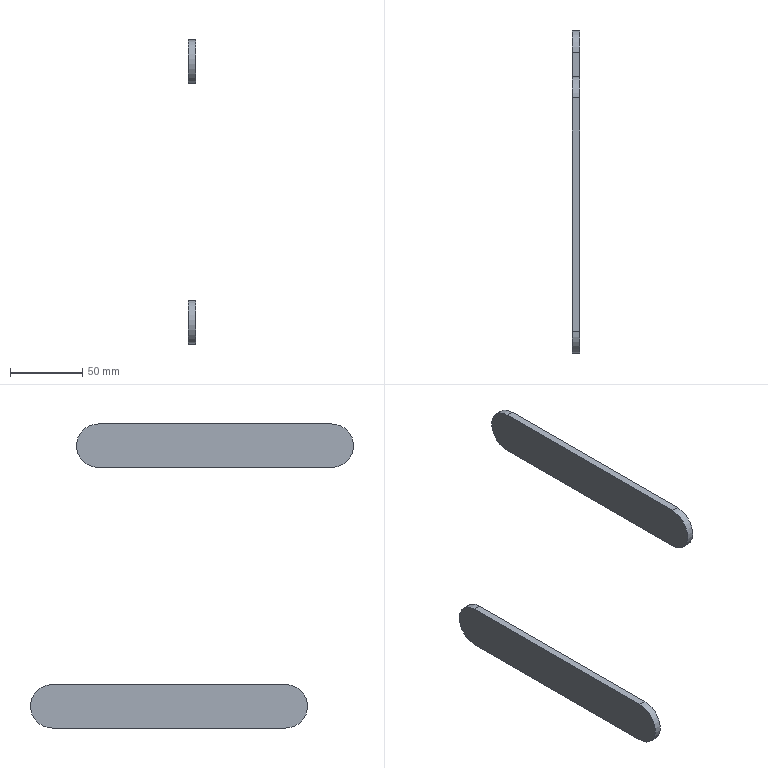Part | NX | features material feeder support 3 | 2 solids | 12 faces | box 5 x 223.069 x 210 mm | volume 55468 mm3 | plane 8 | cylinder 4 | commonest cylinder face diameters 30 x4
STEP:
#1=CARTESIAN_POINT('',(343.,522.298,-562.165));
#2=VERTEX_POINT('',#1);
#3=CARTESIAN_POINT('',(343.,360.967,-562.165));
#4=VERTEX_POINT('',#3);
#5=CARTESIAN_POINT('',(343.,522.298,-562.165));
#6=DIRECTION('',(0.,-1.,0.));
#7=VECTOR('',#6,1000.);
#8=LINE('',#5,#7);
#9=EDGE_CURVE('',#2,#4,#8,.T.);
#10=ORIENTED_EDGE('',*,*,#9,.T.);
#11=CARTESIAN_POINT('',(343.,360.967,-532.165));
#12=VERTEX_POINT('',#11);
#13=CARTESIAN_POINT('',(343.,360.967,-547.165));
#14=DIRECTION('',(-1.,0.,0.));
#15=DIRECTION('',(0.,-1.,0.));
#16=AXIS2_PLACEMENT_3D('',#13,#14,#15);
#17=CIRCLE('',#16,15.);
#18=EDGE_CURVE('',#12,#4,#17,.F.);
#19=ORIENTED_EDGE('',*,*,#18,.F.);
#20=CARTESIAN_POINT('',(343.,522.298,-532.165));
#21=VERTEX_POINT('',#20);
#22=CARTESIAN_POINT('',(343.,522.298,-532.165));
#23=DIRECTION('',(0.,1.,0.));
#24=VECTOR('',#23,1000.);
#25=LINE('',#22,#24);
#26=EDGE_CURVE('',#12,#21,#25,.T.);
#27=ORIENTED_EDGE('',*,*,#26,.T.);
#28=CARTESIAN_POINT('',(343.,522.298,-547.165));
#29=DIRECTION('',(-1.,0.,0.));
#30=DIRECTION('',(0.,-1.,0.));
#31=AXIS2_PLACEMENT_3D('',#28,#29,#30);
#32=CIRCLE('',#31,15.);
#33=EDGE_CURVE('',#2,#21,#32,.F.);
#34=ORIENTED_EDGE('',*,*,#33,.F.);
#35=EDGE_LOOP('',(#10,#19,#27,#34));
#36=FACE_BOUND('',#35,.T.);
#37=CARTESIAN_POINT('',(343.,522.298,-547.165));
#38=DIRECTION('',(1.,0.,0.));
#39=DIRECTION('',(0.,1.,0.));
#40=AXIS2_PLACEMENT_3D('',#37,#38,#39);
#41=PLANE('',#40);
#42=ADVANCED_FACE('',(#36),#41,.F.);
#43=CARTESIAN_POINT('',(348.,522.298,-562.165));
#44=VERTEX_POINT('',#43);
#45=CARTESIAN_POINT('',(348.,522.298,-532.165));
#46=VERTEX_POINT('',#45);
#47=CARTESIAN_POINT('',(348.,522.298,-547.165));
#48=DIRECTION('',(-1.,0.,0.));
#49=DIRECTION('',(0.,-1.,0.));
#50=AXIS2_PLACEMENT_3D('',#47,#48,#49);
#51=CIRCLE('',#50,15.);
#52=EDGE_CURVE('',#44,#46,#51,.F.);
#53=ORIENTED_EDGE('',*,*,#52,.F.);
#54=CARTESIAN_POINT('',(348.,522.298,-562.165));
#55=DIRECTION('',(1.,0.,0.));
#56=VECTOR('',#55,1000.);
#57=LINE('',#54,#56);
#58=EDGE_CURVE('',#44,#2,#57,.F.);
#59=ORIENTED_EDGE('',*,*,#58,.T.);
#60=ORIENTED_EDGE('',*,*,#33,.T.);
#61=CARTESIAN_POINT('',(348.,522.298,-532.165));
#62=DIRECTION('',(-1.,0.,0.));
#63=VECTOR('',#62,1000.);
#64=LINE('',#61,#63);
#65=EDGE_CURVE('',#21,#46,#64,.F.);
#66=ORIENTED_EDGE('',*,*,#65,.T.);
#67=EDGE_LOOP('',(#53,#59,#60,#66));
#68=FACE_BOUND('',#67,.T.);
#69=CARTESIAN_POINT('',(348.,522.298,-547.165));
#70=DIRECTION('',(-1.,0.,0.));
#71=DIRECTION('',(0.,-1.,0.));
#72=AXIS2_PLACEMENT_3D('',#69,#70,#71);
#73=CYLINDRICAL_SURFACE('',#72,15.);
#74=ADVANCED_FACE('',(#68),#73,.T.);
#75=CARTESIAN_POINT('',(348.,360.967,-532.165));
#76=VERTEX_POINT('',#75);
#77=CARTESIAN_POINT('',(348.,360.967,-532.165));
#78=DIRECTION('',(-1.,0.,0.));
#79=VECTOR('',#78,1000.);
#80=LINE('',#77,#79);
#81=EDGE_CURVE('',#76,#12,#80,.T.);
#82=ORIENTED_EDGE('',*,*,#81,.F.);
#83=CARTESIAN_POINT('',(348.,522.298,-532.165));
#84=DIRECTION('',(0.,1.,0.));
#85=VECTOR('',#84,1000.);
#86=LINE('',#83,#85);
#87=EDGE_CURVE('',#46,#76,#86,.F.);
#88=ORIENTED_EDGE('',*,*,#87,.F.);
#89=ORIENTED_EDGE('',*,*,#65,.F.);
#90=ORIENTED_EDGE('',*,*,#26,.F.);
#91=EDGE_LOOP('',(#82,#88,#89,#90));
#92=FACE_BOUND('',#91,.T.);
#93=CARTESIAN_POINT('',(348.,522.298,-532.165));
#94=DIRECTION('',(0.,0.,-1.));
#95=DIRECTION('',(-1.,0.,0.));
#96=AXIS2_PLACEMENT_3D('',#93,#94,#95);
#97=PLANE('',#96);
#98=ADVANCED_FACE('',(#92),#97,.F.);
#99=ORIENTED_EDGE('',*,*,#18,.T.);
#100=CARTESIAN_POINT('',(348.,360.967,-562.165));
#101=VERTEX_POINT('',#100);
#102=CARTESIAN_POINT('',(348.,360.967,-562.165));
#103=DIRECTION('',(1.,0.,0.));
#104=VECTOR('',#103,1000.);
#105=LINE('',#102,#104);
#106=EDGE_CURVE('',#4,#101,#105,.T.);
#107=ORIENTED_EDGE('',*,*,#106,.T.);
#108=CARTESIAN_POINT('',(348.,360.967,-547.165));
#109=DIRECTION('',(-1.,0.,0.));
#110=DIRECTION('',(0.,-1.,0.));
#111=AXIS2_PLACEMENT_3D('',#108,#109,#110);
#112=CIRCLE('',#111,15.);
#113=EDGE_CURVE('',#76,#101,#112,.F.);
#114=ORIENTED_EDGE('',*,*,#113,.F.);
#115=ORIENTED_EDGE('',*,*,#81,.T.);
#116=EDGE_LOOP('',(#99,#107,#114,#115));
#117=FACE_BOUND('',#116,.T.);
#118=CARTESIAN_POINT('',(348.,360.967,-547.165));
#119=DIRECTION('',(-1.,0.,0.));
#120=DIRECTION('',(0.,-1.,0.));
#121=AXIS2_PLACEMENT_3D('',#118,#119,#120);
#122=CYLINDRICAL_SURFACE('',#121,15.);
#123=ADVANCED_FACE('',(#117),#122,.T.);
#124=ORIENTED_EDGE('',*,*,#58,.F.);
#125=CARTESIAN_POINT('',(348.,522.298,-562.165));
#126=DIRECTION('',(0.,1.,0.));
#127=VECTOR('',#126,1000.);
#128=LINE('',#125,#127);
#129=EDGE_CURVE('',#101,#44,#128,.T.);
#130=ORIENTED_EDGE('',*,*,#129,.F.);
#131=ORIENTED_EDGE('',*,*,#106,.F.);
#132=ORIENTED_EDGE('',*,*,#9,.F.);
#133=EDGE_LOOP('',(#124,#130,#131,#132));
#134=FACE_BOUND('',#133,.T.);
#135=CARTESIAN_POINT('',(348.,522.298,-562.165));
#136=DIRECTION('',(0.,0.,1.));
#137=DIRECTION('',(0.,-1.,0.));
#138=AXIS2_PLACEMENT_3D('',#135,#136,#137);
#139=PLANE('',#138);
#140=ADVANCED_FACE('',(#134),#139,.F.);
#141=ORIENTED_EDGE('',*,*,#113,.T.);
#142=ORIENTED_EDGE('',*,*,#129,.T.);
#143=ORIENTED_EDGE('',*,*,#52,.T.);
#144=ORIENTED_EDGE('',*,*,#87,.T.);
#145=EDGE_LOOP('',(#141,#142,#143,#144));
#146=FACE_BOUND('',#145,.T.);
#147=CARTESIAN_POINT('',(348.,522.298,-547.165));
#148=DIRECTION('',(1.,0.,0.));
#149=DIRECTION('',(0.,1.,0.));
#150=AXIS2_PLACEMENT_3D('',#147,#148,#149);
#151=PLANE('',#150);
#152=ADVANCED_FACE('',(#146),#151,.T.);
#153=CLOSED_SHELL('',(#42,#74,#98,#123,#140,#152));
#154=MANIFOLD_SOLID_BREP('',#153);
#155=CARTESIAN_POINT('',(343.,490.559,-382.165));
#156=VERTEX_POINT('',#155);
#157=CARTESIAN_POINT('',(343.,329.228,-382.165));
#158=VERTEX_POINT('',#157);
#159=CARTESIAN_POINT('',(343.,490.559,-382.165));
#160=DIRECTION('',(0.,-1.,0.));
#161=VECTOR('',#160,1000.);
#162=LINE('',#159,#161);
#163=EDGE_CURVE('',#156,#158,#162,.T.);
#164=ORIENTED_EDGE('',*,*,#163,.T.);
#165=CARTESIAN_POINT('',(343.,329.228,-352.165));
#166=VERTEX_POINT('',#165);
#167=CARTESIAN_POINT('',(343.,329.228,-367.165));
#168=DIRECTION('',(-1.,0.,0.));
#169=DIRECTION('',(0.,-1.,0.));
#170=AXIS2_PLACEMENT_3D('',#167,#168,#169);
#171=CIRCLE('',#170,15.);
#172=EDGE_CURVE('',#166,#158,#171,.F.);
#173=ORIENTED_EDGE('',*,*,#172,.F.);
#174=CARTESIAN_POINT('',(343.,490.559,-352.165));
#175=VERTEX_POINT('',#174);
#176=CARTESIAN_POINT('',(343.,490.559,-352.165));
#177=DIRECTION('',(0.,1.,0.));
#178=VECTOR('',#177,1000.);
#179=LINE('',#176,#178);
#180=EDGE_CURVE('',#166,#175,#179,.T.);
#181=ORIENTED_EDGE('',*,*,#180,.T.);
#182=CARTESIAN_POINT('',(343.,490.559,-367.165));
#183=DIRECTION('',(-1.,0.,0.));
#184=DIRECTION('',(0.,-1.,0.));
#185=AXIS2_PLACEMENT_3D('',#182,#183,#184);
#186=CIRCLE('',#185,15.);
#187=EDGE_CURVE('',#156,#175,#186,.F.);
#188=ORIENTED_EDGE('',*,*,#187,.F.);
#189=EDGE_LOOP('',(#164,#173,#181,#188));
#190=FACE_BOUND('',#189,.T.);
#191=CARTESIAN_POINT('',(343.,490.559,-367.165));
#192=DIRECTION('',(1.,0.,0.));
#193=DIRECTION('',(0.,1.,0.));
#194=AXIS2_PLACEMENT_3D('',#191,#192,#193);
#195=PLANE('',#194);
#196=ADVANCED_FACE('',(#190),#195,.F.);
#197=CARTESIAN_POINT('',(348.,490.559,-382.165));
#198=VERTEX_POINT('',#197);
#199=CARTESIAN_POINT('',(348.,490.559,-352.165));
#200=VERTEX_POINT('',#199);
#201=CARTESIAN_POINT('',(348.,490.559,-367.165));
#202=DIRECTION('',(-1.,0.,0.));
#203=DIRECTION('',(0.,-1.,0.));
#204=AXIS2_PLACEMENT_3D('',#201,#202,#203);
#205=CIRCLE('',#204,15.);
#206=EDGE_CURVE('',#198,#200,#205,.F.);
#207=ORIENTED_EDGE('',*,*,#206,.F.);
#208=CARTESIAN_POINT('',(348.,490.559,-382.165));
#209=DIRECTION('',(1.,0.,0.));
#210=VECTOR('',#209,1000.);
#211=LINE('',#208,#210);
#212=EDGE_CURVE('',#198,#156,#211,.F.);
#213=ORIENTED_EDGE('',*,*,#212,.T.);
#214=ORIENTED_EDGE('',*,*,#187,.T.);
#215=CARTESIAN_POINT('',(348.,490.559,-352.165));
#216=DIRECTION('',(-1.,0.,0.));
#217=VECTOR('',#216,1000.);
#218=LINE('',#215,#217);
#219=EDGE_CURVE('',#175,#200,#218,.F.);
#220=ORIENTED_EDGE('',*,*,#219,.T.);
#221=EDGE_LOOP('',(#207,#213,#214,#220));
#222=FACE_BOUND('',#221,.T.);
#223=CARTESIAN_POINT('',(348.,490.559,-367.165));
#224=DIRECTION('',(-1.,0.,0.));
#225=DIRECTION('',(0.,-1.,0.));
#226=AXIS2_PLACEMENT_3D('',#223,#224,#225);
#227=CYLINDRICAL_SURFACE('',#226,15.);
#228=ADVANCED_FACE('',(#222),#227,.T.);
#229=CARTESIAN_POINT('',(348.,329.228,-352.165));
#230=VERTEX_POINT('',#229);
#231=CARTESIAN_POINT('',(348.,329.228,-352.165));
#232=DIRECTION('',(-1.,0.,0.));
#233=VECTOR('',#232,1000.);
#234=LINE('',#231,#233);
#235=EDGE_CURVE('',#230,#166,#234,.T.);
#236=ORIENTED_EDGE('',*,*,#235,.F.);
#237=CARTESIAN_POINT('',(348.,490.559,-352.165));
#238=DIRECTION('',(0.,1.,0.));
#239=VECTOR('',#238,1000.);
#240=LINE('',#237,#239);
#241=EDGE_CURVE('',#200,#230,#240,.F.);
#242=ORIENTED_EDGE('',*,*,#241,.F.);
#243=ORIENTED_EDGE('',*,*,#219,.F.);
#244=ORIENTED_EDGE('',*,*,#180,.F.);
#245=EDGE_LOOP('',(#236,#242,#243,#244));
#246=FACE_BOUND('',#245,.T.);
#247=CARTESIAN_POINT('',(348.,490.559,-352.165));
#248=DIRECTION('',(0.,0.,-1.));
#249=DIRECTION('',(-1.,0.,0.));
#250=AXIS2_PLACEMENT_3D('',#247,#248,#249);
#251=PLANE('',#250);
#252=ADVANCED_FACE('',(#246),#251,.F.);
#253=ORIENTED_EDGE('',*,*,#172,.T.);
#254=CARTESIAN_POINT('',(348.,329.228,-382.165));
#255=VERTEX_POINT('',#254);
#256=CARTESIAN_POINT('',(348.,329.228,-382.165));
#257=DIRECTION('',(1.,0.,0.));
#258=VECTOR('',#257,1000.);
#259=LINE('',#256,#258);
#260=EDGE_CURVE('',#158,#255,#259,.T.);
#261=ORIENTED_EDGE('',*,*,#260,.T.);
#262=CARTESIAN_POINT('',(348.,329.228,-367.165));
#263=DIRECTION('',(-1.,0.,0.));
#264=DIRECTION('',(0.,-1.,0.));
#265=AXIS2_PLACEMENT_3D('',#262,#263,#264);
#266=CIRCLE('',#265,15.);
#267=EDGE_CURVE('',#230,#255,#266,.F.);
#268=ORIENTED_EDGE('',*,*,#267,.F.);
#269=ORIENTED_EDGE('',*,*,#235,.T.);
#270=EDGE_LOOP('',(#253,#261,#268,#269));
#271=FACE_BOUND('',#270,.T.);
#272=CARTESIAN_POINT('',(348.,329.228,-367.165));
#273=DIRECTION('',(-1.,0.,0.));
#274=DIRECTION('',(0.,-1.,0.));
#275=AXIS2_PLACEMENT_3D('',#272,#273,#274);
#276=CYLINDRICAL_SURFACE('',#275,15.);
#277=ADVANCED_FACE('',(#271),#276,.T.);
#278=ORIENTED_EDGE('',*,*,#212,.F.);
#279=CARTESIAN_POINT('',(348.,490.559,-382.165));
#280=DIRECTION('',(0.,1.,0.));
#281=VECTOR('',#280,1000.);
#282=LINE('',#279,#281);
#283=EDGE_CURVE('',#255,#198,#282,.T.);
#284=ORIENTED_EDGE('',*,*,#283,.F.);
#285=ORIENTED_EDGE('',*,*,#260,.F.);
#286=ORIENTED_EDGE('',*,*,#163,.F.);
#287=EDGE_LOOP('',(#278,#284,#285,#286));
#288=FACE_BOUND('',#287,.T.);
#289=CARTESIAN_POINT('',(348.,490.559,-382.165));
#290=DIRECTION('',(0.,0.,1.));
#291=DIRECTION('',(0.,-1.,0.));
#292=AXIS2_PLACEMENT_3D('',#289,#290,#291);
#293=PLANE('',#292);
#294=ADVANCED_FACE('',(#288),#293,.F.);
#295=ORIENTED_EDGE('',*,*,#267,.T.);
#296=ORIENTED_EDGE('',*,*,#283,.T.);
#297=ORIENTED_EDGE('',*,*,#206,.T.);
#298=ORIENTED_EDGE('',*,*,#241,.T.);
#299=EDGE_LOOP('',(#295,#296,#297,#298));
#300=FACE_BOUND('',#299,.T.);
#301=CARTESIAN_POINT('',(348.,490.559,-367.165));
#302=DIRECTION('',(1.,0.,0.));
#303=DIRECTION('',(0.,1.,0.));
#304=AXIS2_PLACEMENT_3D('',#301,#302,#303);
#305=PLANE('',#304);
#306=ADVANCED_FACE('',(#300),#305,.T.);
#307=CLOSED_SHELL('',(#196,#228,#252,#277,#294,#306));
#308=MANIFOLD_SOLID_BREP('',#307);
#309=(LENGTH_UNIT()NAMED_UNIT(*)SI_UNIT(.MILLI.,.METRE.));
#310=UNCERTAINTY_MEASURE_WITH_UNIT(LENGTH_MEASURE(0.00001),#309,'','');
#311=(NAMED_UNIT(*)PLANE_ANGLE_UNIT()SI_UNIT($,.RADIAN.));
#312=(NAMED_UNIT(*)SI_UNIT($,.STERADIAN.)SOLID_ANGLE_UNIT());
#313=(GEOMETRIC_REPRESENTATION_CONTEXT(3)GLOBAL_UNCERTAINTY_ASSIGNED_CONTEXT((#310))GLOBAL_UNIT_ASSIGNED_CONTEXT((#309,#311,#312))REPRESENTATION_CONTEXT('',''));
#314=ADVANCED_BREP_SHAPE_REPRESENTATION('',(#154,#308),#313);